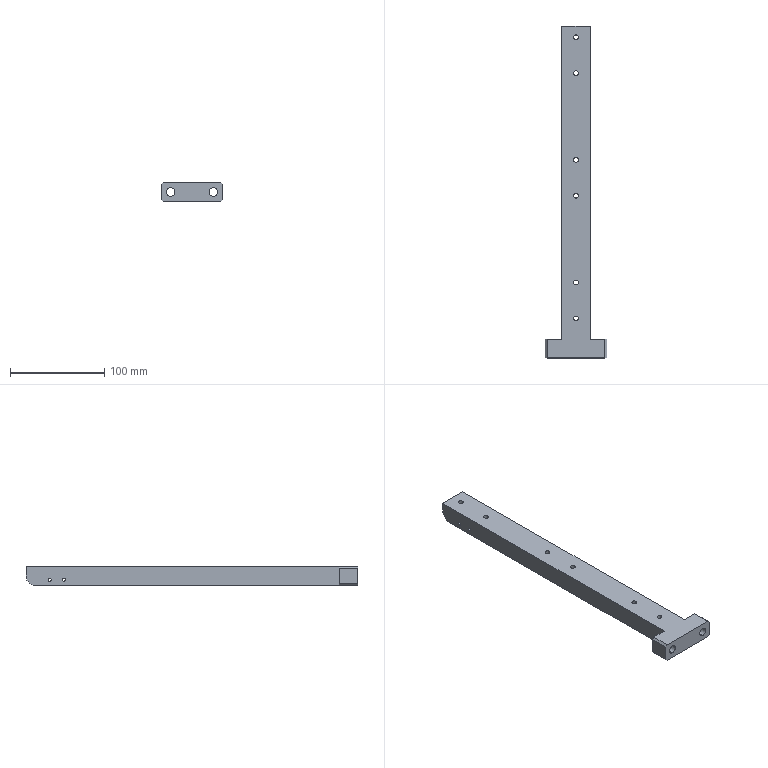Part | SolidWorks | features HoleWzd 3, Chamfer 1, Extrusion 1, Fillet 1, LPattern 1 | 1 solid | 35 faces | box 65 x 352 x 20 mm | volume 218982 mm3 | cylinder 21 | plane 14 | commonest cylinder face diameters 5 x12 3.3 x4 9 x4 20 x1
STEP:
#1=CARTESIAN_POINT('',(-2.5,302.,0.));
#2=VERTEX_POINT('',#1);
#3=CARTESIAN_POINT('',(2.5,302.,0.));
#4=VERTEX_POINT('',#3);
#5=CARTESIAN_POINT('',(0.,302.,0.));
#6=DIRECTION('',(0.,0.,1.));
#7=DIRECTION('',(1.,0.,0.));
#8=AXIS2_PLACEMENT_3D('',#5,#6,#7);
#9=CIRCLE('',#8,2.5);
#10=EDGE_CURVE('',#2,#4,#9,.T.);
#11=ORIENTED_EDGE('',*,*,#10,.F.);
#12=CARTESIAN_POINT('',(-2.5,302.,20.));
#13=VERTEX_POINT('',#12);
#14=CARTESIAN_POINT('',(-2.5,302.,20.));
#15=DIRECTION('',(0.,0.,1.));
#16=VECTOR('',#15,1000.);
#17=LINE('',#14,#16);
#18=EDGE_CURVE('',#2,#13,#17,.T.);
#19=ORIENTED_EDGE('',*,*,#18,.T.);
#20=CARTESIAN_POINT('',(2.5,302.,20.));
#21=VERTEX_POINT('',#20);
#22=CARTESIAN_POINT('',(0.,302.,20.));
#23=DIRECTION('',(0.,0.,1.));
#24=DIRECTION('',(1.,0.,0.));
#25=AXIS2_PLACEMENT_3D('',#22,#23,#24);
#26=CIRCLE('',#25,2.5);
#27=EDGE_CURVE('',#13,#21,#26,.T.);
#28=ORIENTED_EDGE('',*,*,#27,.T.);
#29=CARTESIAN_POINT('',(2.5,302.,20.));
#30=DIRECTION('',(0.,0.,1.));
#31=VECTOR('',#30,1000.);
#32=LINE('',#29,#31);
#33=EDGE_CURVE('',#4,#21,#32,.T.);
#34=ORIENTED_EDGE('',*,*,#33,.F.);
#35=EDGE_LOOP('',(#11,#19,#28,#34));
#36=FACE_OUTER_BOUND('',#35,.T.);
#37=CARTESIAN_POINT('',(0.,302.,20.));
#38=DIRECTION('',(0.,0.,1.));
#39=DIRECTION('',(1.,0.,0.));
#40=AXIS2_PLACEMENT_3D('',#37,#38,#39);
#41=CYLINDRICAL_SURFACE('',#40,2.5);
#42=ADVANCED_FACE('',(#36),#41,.F.);
#43=CARTESIAN_POINT('',(-2.5,172.,0.));
#44=VERTEX_POINT('',#43);
#45=CARTESIAN_POINT('',(2.5,172.,0.));
#46=VERTEX_POINT('',#45);
#47=CARTESIAN_POINT('',(0.,172.,0.));
#48=DIRECTION('',(0.,0.,1.));
#49=DIRECTION('',(1.,0.,0.));
#50=AXIS2_PLACEMENT_3D('',#47,#48,#49);
#51=CIRCLE('',#50,2.5);
#52=EDGE_CURVE('',#44,#46,#51,.T.);
#53=ORIENTED_EDGE('',*,*,#52,.F.);
#54=CARTESIAN_POINT('',(-2.5,172.,20.));
#55=VERTEX_POINT('',#54);
#56=CARTESIAN_POINT('',(-2.5,172.,20.));
#57=DIRECTION('',(0.,0.,1.));
#58=VECTOR('',#57,1000.);
#59=LINE('',#56,#58);
#60=EDGE_CURVE('',#44,#55,#59,.T.);
#61=ORIENTED_EDGE('',*,*,#60,.T.);
#62=CARTESIAN_POINT('',(2.5,172.,20.));
#63=VERTEX_POINT('',#62);
#64=CARTESIAN_POINT('',(0.,172.,20.));
#65=DIRECTION('',(0.,0.,1.));
#66=DIRECTION('',(1.,0.,0.));
#67=AXIS2_PLACEMENT_3D('',#64,#65,#66);
#68=CIRCLE('',#67,2.5);
#69=EDGE_CURVE('',#55,#63,#68,.T.);
#70=ORIENTED_EDGE('',*,*,#69,.T.);
#71=CARTESIAN_POINT('',(2.5,172.,20.));
#72=DIRECTION('',(0.,0.,1.));
#73=VECTOR('',#72,1000.);
#74=LINE('',#71,#73);
#75=EDGE_CURVE('',#46,#63,#74,.T.);
#76=ORIENTED_EDGE('',*,*,#75,.F.);
#77=EDGE_LOOP('',(#53,#61,#70,#76));
#78=FACE_OUTER_BOUND('',#77,.T.);
#79=CARTESIAN_POINT('',(0.,172.,20.));
#80=DIRECTION('',(0.,0.,1.));
#81=DIRECTION('',(1.,0.,0.));
#82=AXIS2_PLACEMENT_3D('',#79,#80,#81);
#83=CYLINDRICAL_SURFACE('',#82,2.5);
#84=ADVANCED_FACE('',(#78),#83,.F.);
#85=CARTESIAN_POINT('',(-2.5,42.,0.));
#86=VERTEX_POINT('',#85);
#87=CARTESIAN_POINT('',(2.5,42.,0.));
#88=VERTEX_POINT('',#87);
#89=CARTESIAN_POINT('',(0.,42.,0.));
#90=DIRECTION('',(0.,0.,1.));
#91=DIRECTION('',(1.,0.,0.));
#92=AXIS2_PLACEMENT_3D('',#89,#90,#91);
#93=CIRCLE('',#92,2.5);
#94=EDGE_CURVE('',#86,#88,#93,.T.);
#95=ORIENTED_EDGE('',*,*,#94,.F.);
#96=CARTESIAN_POINT('',(-2.5,42.,20.));
#97=VERTEX_POINT('',#96);
#98=CARTESIAN_POINT('',(-2.5,42.,20.));
#99=DIRECTION('',(0.,0.,1.));
#100=VECTOR('',#99,1000.);
#101=LINE('',#98,#100);
#102=EDGE_CURVE('',#86,#97,#101,.T.);
#103=ORIENTED_EDGE('',*,*,#102,.T.);
#104=CARTESIAN_POINT('',(2.5,42.,20.));
#105=VERTEX_POINT('',#104);
#106=CARTESIAN_POINT('',(0.,42.,20.));
#107=DIRECTION('',(0.,0.,1.));
#108=DIRECTION('',(1.,0.,0.));
#109=AXIS2_PLACEMENT_3D('',#106,#107,#108);
#110=CIRCLE('',#109,2.5);
#111=EDGE_CURVE('',#97,#105,#110,.T.);
#112=ORIENTED_EDGE('',*,*,#111,.T.);
#113=CARTESIAN_POINT('',(2.5,42.,20.));
#114=DIRECTION('',(0.,0.,1.));
#115=VECTOR('',#114,1000.);
#116=LINE('',#113,#115);
#117=EDGE_CURVE('',#88,#105,#116,.T.);
#118=ORIENTED_EDGE('',*,*,#117,.F.);
#119=EDGE_LOOP('',(#95,#103,#112,#118));
#120=FACE_OUTER_BOUND('',#119,.T.);
#121=CARTESIAN_POINT('',(0.,42.,20.));
#122=DIRECTION('',(0.,0.,1.));
#123=DIRECTION('',(1.,0.,0.));
#124=AXIS2_PLACEMENT_3D('',#121,#122,#123);
#125=CYLINDRICAL_SURFACE('',#124,2.5);
#126=ADVANCED_FACE('',(#120),#125,.F.);
#127=CARTESIAN_POINT('',(15.,327.,4.35));
#128=VERTEX_POINT('',#127);
#129=CARTESIAN_POINT('',(15.,327.,7.65));
#130=VERTEX_POINT('',#129);
#131=CARTESIAN_POINT('',(15.,327.,6.));
#132=DIRECTION('',(-1.,0.,0.));
#133=DIRECTION('',(0.,-1.,0.));
#134=AXIS2_PLACEMENT_3D('',#131,#132,#133);
#135=CIRCLE('',#134,1.65);
#136=EDGE_CURVE('',#128,#130,#135,.T.);
#137=ORIENTED_EDGE('',*,*,#136,.F.);
#138=CARTESIAN_POINT('',(-15.,327.,4.35));
#139=VERTEX_POINT('',#138);
#140=CARTESIAN_POINT('',(-15.,327.,4.35));
#141=DIRECTION('',(-1.,0.,0.));
#142=VECTOR('',#141,1000.);
#143=LINE('',#140,#142);
#144=EDGE_CURVE('',#128,#139,#143,.T.);
#145=ORIENTED_EDGE('',*,*,#144,.T.);
#146=CARTESIAN_POINT('',(-15.,327.,7.65));
#147=VERTEX_POINT('',#146);
#148=CARTESIAN_POINT('',(-15.,327.,6.));
#149=DIRECTION('',(-1.,0.,0.));
#150=DIRECTION('',(0.,0.,1.));
#151=AXIS2_PLACEMENT_3D('',#148,#149,#150);
#152=CIRCLE('',#151,1.65);
#153=EDGE_CURVE('',#139,#147,#152,.T.);
#154=ORIENTED_EDGE('',*,*,#153,.T.);
#155=CARTESIAN_POINT('',(-15.,327.,7.65));
#156=DIRECTION('',(-1.,0.,0.));
#157=VECTOR('',#156,1000.);
#158=LINE('',#155,#157);
#159=EDGE_CURVE('',#130,#147,#158,.T.);
#160=ORIENTED_EDGE('',*,*,#159,.F.);
#161=EDGE_LOOP('',(#137,#145,#154,#160));
#162=FACE_OUTER_BOUND('',#161,.T.);
#163=CARTESIAN_POINT('',(-15.,327.,6.));
#164=DIRECTION('',(-1.,0.,0.));
#165=DIRECTION('',(0.,0.,1.));
#166=AXIS2_PLACEMENT_3D('',#163,#164,#165);
#167=CYLINDRICAL_SURFACE('',#166,1.65);
#168=ADVANCED_FACE('',(#162),#167,.F.);
#169=CARTESIAN_POINT('',(15.,312.,4.35));
#170=VERTEX_POINT('',#169);
#171=CARTESIAN_POINT('',(15.,312.,7.65));
#172=VERTEX_POINT('',#171);
#173=CARTESIAN_POINT('',(15.,312.,6.));
#174=DIRECTION('',(-1.,0.,0.));
#175=DIRECTION('',(0.,-1.,0.));
#176=AXIS2_PLACEMENT_3D('',#173,#174,#175);
#177=CIRCLE('',#176,1.65);
#178=EDGE_CURVE('',#170,#172,#177,.T.);
#179=ORIENTED_EDGE('',*,*,#178,.F.);
#180=CARTESIAN_POINT('',(-15.,312.,4.35));
#181=VERTEX_POINT('',#180);
#182=CARTESIAN_POINT('',(-15.,312.,4.35));
#183=DIRECTION('',(-1.,0.,0.));
#184=VECTOR('',#183,1000.);
#185=LINE('',#182,#184);
#186=EDGE_CURVE('',#170,#181,#185,.T.);
#187=ORIENTED_EDGE('',*,*,#186,.T.);
#188=CARTESIAN_POINT('',(-15.,312.,7.65));
#189=VERTEX_POINT('',#188);
#190=CARTESIAN_POINT('',(-15.,312.,6.));
#191=DIRECTION('',(-1.,0.,0.));
#192=DIRECTION('',(0.,0.,1.));
#193=AXIS2_PLACEMENT_3D('',#190,#191,#192);
#194=CIRCLE('',#193,1.65);
#195=EDGE_CURVE('',#181,#189,#194,.T.);
#196=ORIENTED_EDGE('',*,*,#195,.T.);
#197=CARTESIAN_POINT('',(-15.,312.,7.65));
#198=DIRECTION('',(-1.,0.,0.));
#199=VECTOR('',#198,1000.);
#200=LINE('',#197,#199);
#201=EDGE_CURVE('',#172,#189,#200,.T.);
#202=ORIENTED_EDGE('',*,*,#201,.F.);
#203=EDGE_LOOP('',(#179,#187,#196,#202));
#204=FACE_OUTER_BOUND('',#203,.T.);
#205=CARTESIAN_POINT('',(-15.,312.,6.));
#206=DIRECTION('',(-1.,0.,0.));
#207=DIRECTION('',(0.,0.,1.));
#208=AXIS2_PLACEMENT_3D('',#205,#206,#207);
#209=CYLINDRICAL_SURFACE('',#208,1.65);
#210=ADVANCED_FACE('',(#204),#209,.F.);
#211=CARTESIAN_POINT('',(-2.5,340.,0.));
#212=VERTEX_POINT('',#211);
#213=CARTESIAN_POINT('',(2.5,340.,0.));
#214=VERTEX_POINT('',#213);
#215=CARTESIAN_POINT('',(0.,340.,0.));
#216=DIRECTION('',(0.,0.,1.));
#217=DIRECTION('',(1.,0.,0.));
#218=AXIS2_PLACEMENT_3D('',#215,#216,#217);
#219=CIRCLE('',#218,2.5);
#220=EDGE_CURVE('',#212,#214,#219,.T.);
#221=ORIENTED_EDGE('',*,*,#220,.F.);
#222=CARTESIAN_POINT('',(-2.5,340.,20.));
#223=VERTEX_POINT('',#222);
#224=CARTESIAN_POINT('',(-2.5,340.,20.));
#225=DIRECTION('',(0.,0.,1.));
#226=VECTOR('',#225,1000.);
#227=LINE('',#224,#226);
#228=EDGE_CURVE('',#212,#223,#227,.T.);
#229=ORIENTED_EDGE('',*,*,#228,.T.);
#230=CARTESIAN_POINT('',(2.5,340.,20.));
#231=VERTEX_POINT('',#230);
#232=CARTESIAN_POINT('',(0.,340.,20.));
#233=DIRECTION('',(0.,0.,1.));
#234=DIRECTION('',(1.,0.,0.));
#235=AXIS2_PLACEMENT_3D('',#232,#233,#234);
#236=CIRCLE('',#235,2.5);
#237=EDGE_CURVE('',#223,#231,#236,.T.);
#238=ORIENTED_EDGE('',*,*,#237,.T.);
#239=CARTESIAN_POINT('',(2.5,340.,20.));
#240=DIRECTION('',(0.,0.,1.));
#241=VECTOR('',#240,1000.);
#242=LINE('',#239,#241);
#243=EDGE_CURVE('',#214,#231,#242,.T.);
#244=ORIENTED_EDGE('',*,*,#243,.F.);
#245=EDGE_LOOP('',(#221,#229,#238,#244));
#246=FACE_OUTER_BOUND('',#245,.T.);
#247=CARTESIAN_POINT('',(0.,340.,20.));
#248=DIRECTION('',(0.,0.,1.));
#249=DIRECTION('',(1.,0.,0.));
#250=AXIS2_PLACEMENT_3D('',#247,#248,#249);
#251=CYLINDRICAL_SURFACE('',#250,2.5);
#252=ADVANCED_FACE('',(#246),#251,.F.);
#253=CARTESIAN_POINT('',(-2.5,210.,0.));
#254=VERTEX_POINT('',#253);
#255=CARTESIAN_POINT('',(2.5,210.,0.));
#256=VERTEX_POINT('',#255);
#257=CARTESIAN_POINT('',(0.,210.,0.));
#258=DIRECTION('',(0.,0.,1.));
#259=DIRECTION('',(1.,0.,0.));
#260=AXIS2_PLACEMENT_3D('',#257,#258,#259);
#261=CIRCLE('',#260,2.5);
#262=EDGE_CURVE('',#254,#256,#261,.T.);
#263=ORIENTED_EDGE('',*,*,#262,.F.);
#264=CARTESIAN_POINT('',(-2.5,210.,20.));
#265=VERTEX_POINT('',#264);
#266=CARTESIAN_POINT('',(-2.5,210.,20.));
#267=DIRECTION('',(0.,0.,1.));
#268=VECTOR('',#267,1000.);
#269=LINE('',#266,#268);
#270=EDGE_CURVE('',#254,#265,#269,.T.);
#271=ORIENTED_EDGE('',*,*,#270,.T.);
#272=CARTESIAN_POINT('',(2.5,210.,20.));
#273=VERTEX_POINT('',#272);
#274=CARTESIAN_POINT('',(0.,210.,20.));
#275=DIRECTION('',(0.,0.,1.));
#276=DIRECTION('',(1.,0.,0.));
#277=AXIS2_PLACEMENT_3D('',#274,#275,#276);
#278=CIRCLE('',#277,2.5);
#279=EDGE_CURVE('',#265,#273,#278,.T.);
#280=ORIENTED_EDGE('',*,*,#279,.T.);
#281=CARTESIAN_POINT('',(2.5,210.,20.));
#282=DIRECTION('',(0.,0.,1.));
#283=VECTOR('',#282,1000.);
#284=LINE('',#281,#283);
#285=EDGE_CURVE('',#256,#273,#284,.T.);
#286=ORIENTED_EDGE('',*,*,#285,.F.);
#287=EDGE_LOOP('',(#263,#271,#280,#286));
#288=FACE_OUTER_BOUND('',#287,.T.);
#289=CARTESIAN_POINT('',(0.,210.,20.));
#290=DIRECTION('',(0.,0.,1.));
#291=DIRECTION('',(1.,0.,0.));
#292=AXIS2_PLACEMENT_3D('',#289,#290,#291);
#293=CYLINDRICAL_SURFACE('',#292,2.5);
#294=ADVANCED_FACE('',(#288),#293,.F.);
#295=CARTESIAN_POINT('',(-2.5,80.,0.));
#296=VERTEX_POINT('',#295);
#297=CARTESIAN_POINT('',(2.5,80.,0.));
#298=VERTEX_POINT('',#297);
#299=CARTESIAN_POINT('',(0.,80.,0.));
#300=DIRECTION('',(0.,0.,1.));
#301=DIRECTION('',(1.,0.,0.));
#302=AXIS2_PLACEMENT_3D('',#299,#300,#301);
#303=CIRCLE('',#302,2.5);
#304=EDGE_CURVE('',#296,#298,#303,.T.);
#305=ORIENTED_EDGE('',*,*,#304,.F.);
#306=CARTESIAN_POINT('',(-2.5,80.,20.));
#307=VERTEX_POINT('',#306);
#308=CARTESIAN_POINT('',(-2.5,80.,20.));
#309=DIRECTION('',(0.,0.,1.));
#310=VECTOR('',#309,1000.);
#311=LINE('',#308,#310);
#312=EDGE_CURVE('',#296,#307,#311,.T.);
#313=ORIENTED_EDGE('',*,*,#312,.T.);
#314=CARTESIAN_POINT('',(2.5,80.,20.));
#315=VERTEX_POINT('',#314);
#316=CARTESIAN_POINT('',(0.,80.,20.));
#317=DIRECTION('',(0.,0.,1.));
#318=DIRECTION('',(1.,0.,0.));
#319=AXIS2_PLACEMENT_3D('',#316,#317,#318);
#320=CIRCLE('',#319,2.5);
#321=EDGE_CURVE('',#307,#315,#320,.T.);
#322=ORIENTED_EDGE('',*,*,#321,.T.);
#323=CARTESIAN_POINT('',(2.5,80.,20.));
#324=DIRECTION('',(0.,0.,1.));
#325=VECTOR('',#324,1000.);
#326=LINE('',#323,#325);
#327=EDGE_CURVE('',#298,#315,#326,.T.);
#328=ORIENTED_EDGE('',*,*,#327,.F.);
#329=EDGE_LOOP('',(#305,#313,#322,#328));
#330=FACE_OUTER_BOUND('',#329,.T.);
#331=CARTESIAN_POINT('',(0.,80.,20.));
#332=DIRECTION('',(0.,0.,1.));
#333=DIRECTION('',(1.,0.,0.));
#334=AXIS2_PLACEMENT_3D('',#331,#332,#333);
#335=CYLINDRICAL_SURFACE('',#334,2.5);
#336=ADVANCED_FACE('',(#330),#335,.F.);
#337=CARTESIAN_POINT('',(22.5,0.,5.5));
#338=VERTEX_POINT('',#337);
#339=CARTESIAN_POINT('',(22.5,0.,14.5));
#340=VERTEX_POINT('',#339);
#341=CARTESIAN_POINT('',(22.5,0.,10.));
#342=DIRECTION('',(0.,1.,0.));
#343=DIRECTION('',(0.,0.,1.));
#344=AXIS2_PLACEMENT_3D('',#341,#342,#343);
#345=CIRCLE('',#344,4.5);
#346=EDGE_CURVE('',#338,#340,#345,.T.);
#347=ORIENTED_EDGE('',*,*,#346,.F.);
#348=CARTESIAN_POINT('',(22.5,20.,5.5));
#349=VERTEX_POINT('',#348);
#350=CARTESIAN_POINT('',(22.5,20.,5.5));
#351=DIRECTION('',(0.,1.,0.));
#352=VECTOR('',#351,1000.);
#353=LINE('',#350,#352);
#354=EDGE_CURVE('',#338,#349,#353,.T.);
#355=ORIENTED_EDGE('',*,*,#354,.T.);
#356=CARTESIAN_POINT('',(22.5,20.,14.5));
#357=VERTEX_POINT('',#356);
#358=CARTESIAN_POINT('',(22.5,20.,10.));
#359=DIRECTION('',(0.,1.,0.));
#360=DIRECTION('',(0.,0.,1.));
#361=AXIS2_PLACEMENT_3D('',#358,#359,#360);
#362=CIRCLE('',#361,4.5);
#363=EDGE_CURVE('',#349,#357,#362,.T.);
#364=ORIENTED_EDGE('',*,*,#363,.T.);
#365=CARTESIAN_POINT('',(22.5,20.,14.5));
#366=DIRECTION('',(0.,1.,0.));
#367=VECTOR('',#366,1000.);
#368=LINE('',#365,#367);
#369=EDGE_CURVE('',#340,#357,#368,.T.);
#370=ORIENTED_EDGE('',*,*,#369,.F.);
#371=EDGE_LOOP('',(#347,#355,#364,#370));
#372=FACE_OUTER_BOUND('',#371,.T.);
#373=CARTESIAN_POINT('',(22.5,20.,10.));
#374=DIRECTION('',(0.,1.,0.));
#375=DIRECTION('',(0.,0.,1.));
#376=AXIS2_PLACEMENT_3D('',#373,#374,#375);
#377=CYLINDRICAL_SURFACE('',#376,4.5);
#378=ADVANCED_FACE('',(#372),#377,.F.);
#379=CARTESIAN_POINT('',(-22.5,0.,5.5));
#380=VERTEX_POINT('',#379);
#381=CARTESIAN_POINT('',(-22.5,0.,14.5));
#382=VERTEX_POINT('',#381);
#383=CARTESIAN_POINT('',(-22.5,0.,10.));
#384=DIRECTION('',(0.,1.,0.));
#385=DIRECTION('',(0.,0.,1.));
#386=AXIS2_PLACEMENT_3D('',#383,#384,#385);
#387=CIRCLE('',#386,4.5);
#388=EDGE_CURVE('',#380,#382,#387,.T.);
#389=ORIENTED_EDGE('',*,*,#388,.F.);
#390=CARTESIAN_POINT('',(-22.5,20.,5.5));
#391=VERTEX_POINT('',#390);
#392=CARTESIAN_POINT('',(-22.5,20.,5.5));
#393=DIRECTION('',(0.,1.,0.));
#394=VECTOR('',#393,1000.);
#395=LINE('',#392,#394);
#396=EDGE_CURVE('',#380,#391,#395,.T.);
#397=ORIENTED_EDGE('',*,*,#396,.T.);
#398=CARTESIAN_POINT('',(-22.5,20.,14.5));
#399=VERTEX_POINT('',#398);
#400=CARTESIAN_POINT('',(-22.5,20.,10.));
#401=DIRECTION('',(0.,1.,0.));
#402=DIRECTION('',(0.,0.,1.));
#403=AXIS2_PLACEMENT_3D('',#400,#401,#402);
#404=CIRCLE('',#403,4.5);
#405=EDGE_CURVE('',#391,#399,#404,.T.);
#406=ORIENTED_EDGE('',*,*,#405,.T.);
#407=CARTESIAN_POINT('',(-22.5,20.,14.5));
#408=DIRECTION('',(0.,1.,0.));
#409=VECTOR('',#408,1000.);
#410=LINE('',#407,#409);
#411=EDGE_CURVE('',#382,#399,#410,.T.);
#412=ORIENTED_EDGE('',*,*,#411,.F.);
#413=EDGE_LOOP('',(#389,#397,#406,#412));
#414=FACE_OUTER_BOUND('',#413,.T.);
#415=CARTESIAN_POINT('',(-22.5,20.,10.));
#416=DIRECTION('',(0.,1.,0.));
#417=DIRECTION('',(0.,0.,1.));
#418=AXIS2_PLACEMENT_3D('',#415,#416,#417);
#419=CYLINDRICAL_SURFACE('',#418,4.5);
#420=ADVANCED_FACE('',(#414),#419,.F.);
#421=CARTESIAN_POINT('',(0.,302.,0.));
#422=DIRECTION('',(0.,0.,1.));
#423=DIRECTION('',(1.,0.,0.));
#424=AXIS2_PLACEMENT_3D('',#421,#422,#423);
#425=CIRCLE('',#424,2.5);
#426=EDGE_CURVE('',#4,#2,#425,.T.);
#427=ORIENTED_EDGE('',*,*,#426,.T.);
#428=ORIENTED_EDGE('',*,*,#10,.T.);
#429=EDGE_LOOP('',(#427,#428));
#430=FACE_BOUND('',#429,.T.);
#431=CARTESIAN_POINT('',(0.,172.,0.));
#432=DIRECTION('',(0.,0.,1.));
#433=DIRECTION('',(1.,0.,0.));
#434=AXIS2_PLACEMENT_3D('',#431,#432,#433);
#435=CIRCLE('',#434,2.5);
#436=EDGE_CURVE('',#46,#44,#435,.T.);
#437=ORIENTED_EDGE('',*,*,#436,.T.);
#438=ORIENTED_EDGE('',*,*,#52,.T.);
#439=EDGE_LOOP('',(#437,#438));
#440=FACE_BOUND('',#439,.T.);
#441=CARTESIAN_POINT('',(0.,80.,0.));
#442=DIRECTION('',(0.,0.,1.));
#443=DIRECTION('',(1.,0.,0.));
#444=AXIS2_PLACEMENT_3D('',#441,#442,#443);
#445=CIRCLE('',#444,2.5);
#446=EDGE_CURVE('',#298,#296,#445,.T.);
#447=ORIENTED_EDGE('',*,*,#446,.T.);
#448=ORIENTED_EDGE('',*,*,#304,.T.);
#449=EDGE_LOOP('',(#447,#448));
#450=FACE_BOUND('',#449,.T.);
#451=CARTESIAN_POINT('',(0.,210.,0.));
#452=DIRECTION('',(0.,0.,1.));
#453=DIRECTION('',(1.,0.,0.));
#454=AXIS2_PLACEMENT_3D('',#451,#452,#453);
#455=CIRCLE('',#454,2.5);
#456=EDGE_CURVE('',#256,#254,#455,.T.);
#457=ORIENTED_EDGE('',*,*,#456,.T.);
#458=ORIENTED_EDGE('',*,*,#262,.T.);
#459=EDGE_LOOP('',(#457,#458));
#460=FACE_BOUND('',#459,.T.);
#461=CARTESIAN_POINT('',(30.5,20.,0.));
#462=VERTEX_POINT('',#461);
#463=CARTESIAN_POINT('',(15.,20.,0.));
#464=VERTEX_POINT('',#463);
#465=CARTESIAN_POINT('',(15.,20.,0.));
#466=DIRECTION('',(-1.,0.,0.));
#467=VECTOR('',#466,1000.);
#468=LINE('',#465,#467);
#469=EDGE_CURVE('',#462,#464,#468,.T.);
#470=ORIENTED_EDGE('',*,*,#469,.F.);
#471=CARTESIAN_POINT('',(30.5,0.,0.));
#472=VERTEX_POINT('',#471);
#473=CARTESIAN_POINT('',(30.5,0.,0.));
#474=DIRECTION('',(0.,-1.,0.));
#475=VECTOR('',#474,1000.);
#476=LINE('',#473,#475);
#477=EDGE_CURVE('',#462,#472,#476,.T.);
#478=ORIENTED_EDGE('',*,*,#477,.T.);
#479=CARTESIAN_POINT('',(-30.5,0.,0.));
#480=VERTEX_POINT('',#479);
#481=CARTESIAN_POINT('',(-32.5,0.,0.));
#482=DIRECTION('',(1.,0.,0.));
#483=VECTOR('',#482,1000.);
#484=LINE('',#481,#483);
#485=EDGE_CURVE('',#480,#472,#484,.T.);
#486=ORIENTED_EDGE('',*,*,#485,.F.);
#487=CARTESIAN_POINT('',(-30.5,20.,0.));
#488=VERTEX_POINT('',#487);
#489=CARTESIAN_POINT('',(-30.5,20.,0.));
#490=DIRECTION('',(0.,1.,0.));
#491=VECTOR('',#490,1000.);
#492=LINE('',#489,#491);
#493=EDGE_CURVE('',#480,#488,#492,.T.);
#494=ORIENTED_EDGE('',*,*,#493,.T.);
#495=CARTESIAN_POINT('',(-15.,20.,0.));
#496=VERTEX_POINT('',#495);
#497=CARTESIAN_POINT('',(-15.,20.,0.));
#498=DIRECTION('',(-1.,0.,0.));
#499=VECTOR('',#498,1000.);
#500=LINE('',#497,#499);
#501=EDGE_CURVE('',#496,#488,#500,.T.);
#502=ORIENTED_EDGE('',*,*,#501,.F.);
#503=CARTESIAN_POINT('',(-15.,342.,0.));
#504=VERTEX_POINT('',#503);
#505=CARTESIAN_POINT('',(-15.,352.,0.));
#506=DIRECTION('',(0.,-1.,0.));
#507=VECTOR('',#506,1000.);
#508=LINE('',#505,#507);
#509=EDGE_CURVE('',#504,#496,#508,.T.);
#510=ORIENTED_EDGE('',*,*,#509,.F.);
#511=CARTESIAN_POINT('',(-1.5,342.,0.));
#512=VERTEX_POINT('',#511);
#513=CARTESIAN_POINT('',(15.,342.,0.));
#514=DIRECTION('',(1.,0.,0.));
#515=VECTOR('',#514,1000.);
#516=LINE('',#513,#515);
#517=EDGE_CURVE('',#504,#512,#516,.T.);
#518=ORIENTED_EDGE('',*,*,#517,.T.);
#519=CARTESIAN_POINT('',(0.,340.,0.));
#520=DIRECTION('',(0.,0.,1.));
#521=DIRECTION('',(1.,0.,0.));
#522=AXIS2_PLACEMENT_3D('',#519,#520,#521);
#523=CIRCLE('',#522,2.5);
#524=EDGE_CURVE('',#512,#212,#523,.T.);
#525=ORIENTED_EDGE('',*,*,#524,.T.);
#526=ORIENTED_EDGE('',*,*,#220,.T.);
#527=CARTESIAN_POINT('',(1.5,342.,0.));
#528=VERTEX_POINT('',#527);
#529=CARTESIAN_POINT('',(0.,340.,0.));
#530=DIRECTION('',(0.,0.,1.));
#531=DIRECTION('',(1.,0.,0.));
#532=AXIS2_PLACEMENT_3D('',#529,#530,#531);
#533=CIRCLE('',#532,2.5);
#534=EDGE_CURVE('',#214,#528,#533,.T.);
#535=ORIENTED_EDGE('',*,*,#534,.T.);
#536=CARTESIAN_POINT('',(15.,342.,0.));
#537=VERTEX_POINT('',#536);
#538=CARTESIAN_POINT('',(15.,342.,0.));
#539=DIRECTION('',(1.,0.,0.));
#540=VECTOR('',#539,1000.);
#541=LINE('',#538,#540);
#542=EDGE_CURVE('',#528,#537,#541,.T.);
#543=ORIENTED_EDGE('',*,*,#542,.T.);
#544=CARTESIAN_POINT('',(15.,352.,0.));
#545=DIRECTION('',(0.,1.,0.));
#546=VECTOR('',#545,1000.);
#547=LINE('',#544,#546);
#548=EDGE_CURVE('',#464,#537,#547,.T.);
#549=ORIENTED_EDGE('',*,*,#548,.F.);
#550=EDGE_LOOP('',(#470,#478,#486,#494,#502,#510,#518,#525,#526,#535,#543,#549));
#551=FACE_OUTER_BOUND('',#550,.T.);
#552=CARTESIAN_POINT('',(0.,42.,0.));
#553=DIRECTION('',(0.,0.,1.));
#554=DIRECTION('',(1.,0.,0.));
#555=AXIS2_PLACEMENT_3D('',#552,#553,#554);
#556=CIRCLE('',#555,2.5);
#557=EDGE_CURVE('',#88,#86,#556,.T.);
#558=ORIENTED_EDGE('',*,*,#557,.T.);
#559=ORIENTED_EDGE('',*,*,#94,.T.);
#560=EDGE_LOOP('',(#558,#559));
#561=FACE_BOUND('',#560,.T.);
#562=CARTESIAN_POINT('',(0.,0.,0.));
#563=DIRECTION('',(0.,0.,-1.));
#564=DIRECTION('',(-1.,0.,0.));
#565=AXIS2_PLACEMENT_3D('',#562,#563,#564);
#566=PLANE('',#565);
#567=ADVANCED_FACE('',(#430,#440,#450,#460,#551,#561),#566,.T.);
#568=CARTESIAN_POINT('',(-15.,327.,6.));
#569=DIRECTION('',(-1.,0.,0.));
#570=DIRECTION('',(0.,0.,1.));
#571=AXIS2_PLACEMENT_3D('',#568,#569,#570);
#572=CIRCLE('',#571,1.65);
#573=EDGE_CURVE('',#147,#139,#572,.T.);
#574=ORIENTED_EDGE('',*,*,#573,.F.);
#575=ORIENTED_EDGE('',*,*,#153,.F.);
#576=EDGE_LOOP('',(#574,#575));
#577=FACE_BOUND('',#576,.T.);
#578=CARTESIAN_POINT('',(-15.,312.,6.));
#579=DIRECTION('',(-1.,0.,0.));
#580=DIRECTION('',(0.,0.,1.));
#581=AXIS2_PLACEMENT_3D('',#578,#579,#580);
#582=CIRCLE('',#581,1.65);
#583=EDGE_CURVE('',#189,#181,#582,.T.);
#584=ORIENTED_EDGE('',*,*,#583,.F.);
#585=ORIENTED_EDGE('',*,*,#195,.F.);
#586=EDGE_LOOP('',(#584,#585));
#587=FACE_BOUND('',#586,.T.);
#588=CARTESIAN_POINT('',(-15.,352.,20.));
#589=VERTEX_POINT('',#588);
#590=CARTESIAN_POINT('',(-15.,352.,10.));
#591=VERTEX_POINT('',#590);
#592=CARTESIAN_POINT('',(-15.,352.,20.));
#593=DIRECTION('',(0.,0.,-1.));
#594=VECTOR('',#593,1000.);
#595=LINE('',#592,#594);
#596=EDGE_CURVE('',#589,#591,#595,.T.);
#597=ORIENTED_EDGE('',*,*,#596,.T.);
#598=CARTESIAN_POINT('',(-15.,342.,10.));
#599=DIRECTION('',(-1.,0.,0.));
#600=DIRECTION('',(0.,1.,0.));
#601=AXIS2_PLACEMENT_3D('',#598,#599,#600);
#602=CIRCLE('',#601,10.);
#603=EDGE_CURVE('',#591,#504,#602,.T.);
#604=ORIENTED_EDGE('',*,*,#603,.T.);
#605=ORIENTED_EDGE('',*,*,#509,.T.);
#606=CARTESIAN_POINT('',(-15.,20.,20.));
#607=VERTEX_POINT('',#606);
#608=CARTESIAN_POINT('',(-15.,20.,20.));
#609=DIRECTION('',(0.,0.,-1.));
#610=VECTOR('',#609,1000.);
#611=LINE('',#608,#610);
#612=EDGE_CURVE('',#607,#496,#611,.T.);
#613=ORIENTED_EDGE('',*,*,#612,.F.);
#614=CARTESIAN_POINT('',(-15.,352.,20.));
#615=DIRECTION('',(0.,-1.,0.));
#616=VECTOR('',#615,1000.);
#617=LINE('',#614,#616);
#618=EDGE_CURVE('',#589,#607,#617,.T.);
#619=ORIENTED_EDGE('',*,*,#618,.F.);
#620=EDGE_LOOP('',(#597,#604,#605,#613,#619));
#621=FACE_OUTER_BOUND('',#620,.T.);
#622=CARTESIAN_POINT('',(-15.,352.,20.));
#623=DIRECTION('',(1.,0.,0.));
#624=DIRECTION('',(0.,1.,0.));
#625=AXIS2_PLACEMENT_3D('',#622,#623,#624);
#626=PLANE('',#625);
#627=ADVANCED_FACE('',(#577,#587,#621),#626,.F.);
#628=CARTESIAN_POINT('',(-22.5,20.,10.));
#629=DIRECTION('',(0.,1.,0.));
#630=DIRECTION('',(0.,0.,1.));
#631=AXIS2_PLACEMENT_3D('',#628,#629,#630);
#632=CIRCLE('',#631,4.5);
#633=EDGE_CURVE('',#399,#391,#632,.T.);
#634=ORIENTED_EDGE('',*,*,#633,.F.);
#635=ORIENTED_EDGE('',*,*,#405,.F.);
#636=EDGE_LOOP('',(#634,#635));
#637=FACE_BOUND('',#636,.T.);
#638=CARTESIAN_POINT('',(-32.5,20.,18.));
#639=VERTEX_POINT('',#638);
#640=CARTESIAN_POINT('',(-32.5,20.,2.));
#641=VERTEX_POINT('',#640);
#642=CARTESIAN_POINT('',(-32.5,20.,20.));
#643=DIRECTION('',(0.,0.,-1.));
#644=VECTOR('',#643,1000.);
#645=LINE('',#642,#644);
#646=EDGE_CURVE('',#639,#641,#645,.T.);
#647=ORIENTED_EDGE('',*,*,#646,.F.);
#648=CARTESIAN_POINT('',(-30.5,20.,20.));
#649=VERTEX_POINT('',#648);
#650=CARTESIAN_POINT('',(-30.5,20.,20.));
#651=DIRECTION('',(0.7071,0.,0.7071));
#652=VECTOR('',#651,1000.);
#653=LINE('',#650,#652);
#654=EDGE_CURVE('',#639,#649,#653,.T.);
#655=ORIENTED_EDGE('',*,*,#654,.T.);
#656=CARTESIAN_POINT('',(-15.,20.,20.));
#657=DIRECTION('',(-1.,0.,0.));
#658=VECTOR('',#657,1000.);
#659=LINE('',#656,#658);
#660=EDGE_CURVE('',#607,#649,#659,.T.);
#661=ORIENTED_EDGE('',*,*,#660,.F.);
#662=ORIENTED_EDGE('',*,*,#612,.T.);
#663=ORIENTED_EDGE('',*,*,#501,.T.);
#664=CARTESIAN_POINT('',(-32.5,20.,2.));
#665=DIRECTION('',(-0.7071,0.,0.7071));
#666=VECTOR('',#665,1000.);
#667=LINE('',#664,#666);
#668=EDGE_CURVE('',#488,#641,#667,.T.);
#669=ORIENTED_EDGE('',*,*,#668,.T.);
#670=EDGE_LOOP('',(#647,#655,#661,#662,#663,#669));
#671=FACE_OUTER_BOUND('',#670,.T.);
#672=CARTESIAN_POINT('',(-15.,20.,20.));
#673=DIRECTION('',(0.,-1.,0.));
#674=DIRECTION('',(1.,0.,0.));
#675=AXIS2_PLACEMENT_3D('',#672,#673,#674);
#676=PLANE('',#675);
#677=ADVANCED_FACE('',(#637,#671),#676,.F.);
#678=CARTESIAN_POINT('',(-32.5,0.,18.));
#679=VERTEX_POINT('',#678);
#680=CARTESIAN_POINT('',(-32.5,0.,2.));
#681=VERTEX_POINT('',#680);
#682=CARTESIAN_POINT('',(-32.5,0.,20.));
#683=DIRECTION('',(0.,0.,-1.));
#684=VECTOR('',#683,1000.);
#685=LINE('',#682,#684);
#686=EDGE_CURVE('',#679,#681,#685,.T.);
#687=ORIENTED_EDGE('',*,*,#686,.F.);
#688=CARTESIAN_POINT('',(-32.5,20.,18.));
#689=DIRECTION('',(0.,1.,0.));
#690=VECTOR('',#689,1000.);
#691=LINE('',#688,#690);
#692=EDGE_CURVE('',#679,#639,#691,.T.);
#693=ORIENTED_EDGE('',*,*,#692,.T.);
#694=ORIENTED_EDGE('',*,*,#646,.T.);
#695=CARTESIAN_POINT('',(-32.5,0.,2.));
#696=DIRECTION('',(0.,-1.,0.));
#697=VECTOR('',#696,1000.);
#698=LINE('',#695,#697);
#699=EDGE_CURVE('',#641,#681,#698,.T.);
#700=ORIENTED_EDGE('',*,*,#699,.T.);
#701=EDGE_LOOP('',(#687,#693,#694,#700));
#702=FACE_OUTER_BOUND('',#701,.T.);
#703=CARTESIAN_POINT('',(-32.5,20.,20.));
#704=DIRECTION('',(1.,0.,0.));
#705=DIRECTION('',(0.,1.,0.));
#706=AXIS2_PLACEMENT_3D('',#703,#704,#705);
#707=PLANE('',#706);
#708=ADVANCED_FACE('',(#702),#707,.F.);
#709=CARTESIAN_POINT('',(22.5,0.,10.));
#710=DIRECTION('',(0.,1.,0.));
#711=DIRECTION('',(0.,0.,1.));
#712=AXIS2_PLACEMENT_3D('',#709,#710,#711);
#713=CIRCLE('',#712,4.5);
#714=EDGE_CURVE('',#340,#338,#713,.T.);
#715=ORIENTED_EDGE('',*,*,#714,.T.);
#716=ORIENTED_EDGE('',*,*,#346,.T.);
#717=EDGE_LOOP('',(#715,#716));
#718=FACE_BOUND('',#717,.T.);
#719=CARTESIAN_POINT('',(-22.5,0.,10.));
#720=DIRECTION('',(0.,1.,0.));
#721=DIRECTION('',(0.,0.,1.));
#722=AXIS2_PLACEMENT_3D('',#719,#720,#721);
#723=CIRCLE('',#722,4.5);
#724=EDGE_CURVE('',#382,#380,#723,.T.);
#725=ORIENTED_EDGE('',*,*,#724,.T.);
#726=ORIENTED_EDGE('',*,*,#388,.T.);
#727=EDGE_LOOP('',(#725,#726));
#728=FACE_BOUND('',#727,.T.);
#729=CARTESIAN_POINT('',(32.5,0.,18.));
#730=VERTEX_POINT('',#729);
#731=CARTESIAN_POINT('',(32.5,0.,2.));
#732=VERTEX_POINT('',#731);
#733=CARTESIAN_POINT('',(32.5,0.,20.));
#734=DIRECTION('',(0.,0.,-1.));
#735=VECTOR('',#734,1000.);
#736=LINE('',#733,#735);
#737=EDGE_CURVE('',#730,#732,#736,.T.);
#738=ORIENTED_EDGE('',*,*,#737,.F.);
#739=CARTESIAN_POINT('',(30.5,0.,20.));
#740=VERTEX_POINT('',#739);
#741=CARTESIAN_POINT('',(30.5,0.,20.));
#742=DIRECTION('',(-0.7071,0.,0.7071));
#743=VECTOR('',#742,1000.);
#744=LINE('',#741,#743);
#745=EDGE_CURVE('',#730,#740,#744,.T.);
#746=ORIENTED_EDGE('',*,*,#745,.T.);
#747=CARTESIAN_POINT('',(-30.5,0.,20.));
#748=VERTEX_POINT('',#747);
#749=CARTESIAN_POINT('',(-32.5,0.,20.));
#750=DIRECTION('',(1.,0.,0.));
#751=VECTOR('',#750,1000.);
#752=LINE('',#749,#751);
#753=EDGE_CURVE('',#748,#740,#752,.T.);
#754=ORIENTED_EDGE('',*,*,#753,.F.);
#755=CARTESIAN_POINT('',(-30.5,0.,20.));
#756=DIRECTION('',(-0.7071,0.,-0.7071));
#757=VECTOR('',#756,1000.);
#758=LINE('',#755,#757);
#759=EDGE_CURVE('',#748,#679,#758,.T.);
#760=ORIENTED_EDGE('',*,*,#759,.T.);
#761=ORIENTED_EDGE('',*,*,#686,.T.);
#762=CARTESIAN_POINT('',(-32.5,0.,2.));
#763=DIRECTION('',(0.7071,0.,-0.7071));
#764=VECTOR('',#763,1000.);
#765=LINE('',#762,#764);
#766=EDGE_CURVE('',#681,#480,#765,.T.);
#767=ORIENTED_EDGE('',*,*,#766,.T.);
#768=ORIENTED_EDGE('',*,*,#485,.T.);
#769=CARTESIAN_POINT('',(32.5,0.,2.));
#770=DIRECTION('',(0.7071,0.,0.7071));
#771=VECTOR('',#770,1000.);
#772=LINE('',#769,#771);
#773=EDGE_CURVE('',#472,#732,#772,.T.);
#774=ORIENTED_EDGE('',*,*,#773,.T.);
#775=EDGE_LOOP('',(#738,#746,#754,#760,#761,#767,#768,#774));
#776=FACE_OUTER_BOUND('',#775,.T.);
#777=CARTESIAN_POINT('',(-32.5,0.,20.));
#778=DIRECTION('',(0.,1.,0.));
#779=DIRECTION('',(0.,0.,1.));
#780=AXIS2_PLACEMENT_3D('',#777,#778,#779);
#781=PLANE('',#780);
#782=ADVANCED_FACE('',(#718,#728,#776),#781,.F.);
#783=CARTESIAN_POINT('',(32.5,20.,18.));
#784=VERTEX_POINT('',#783);
#785=CARTESIAN_POINT('',(32.5,20.,2.));
#786=VERTEX_POINT('',#785);
#787=CARTESIAN_POINT('',(32.5,20.,20.));
#788=DIRECTION('',(0.,0.,-1.));
#789=VECTOR('',#788,1000.);
#790=LINE('',#787,#789);
#791=EDGE_CURVE('',#784,#786,#790,.T.);
#792=ORIENTED_EDGE('',*,*,#791,.F.);
#793=CARTESIAN_POINT('',(32.5,20.,18.));
#794=DIRECTION('',(0.,-1.,0.));
#795=VECTOR('',#794,1000.);
#796=LINE('',#793,#795);
#797=EDGE_CURVE('',#784,#730,#796,.T.);
#798=ORIENTED_EDGE('',*,*,#797,.T.);
#799=ORIENTED_EDGE('',*,*,#737,.T.);
#800=CARTESIAN_POINT('',(32.5,20.,2.));
#801=DIRECTION('',(0.,1.,0.));
#802=VECTOR('',#801,1000.);
#803=LINE('',#800,#802);
#804=EDGE_CURVE('',#732,#786,#803,.T.);
#805=ORIENTED_EDGE('',*,*,#804,.T.);
#806=EDGE_LOOP('',(#792,#798,#799,#805));
#807=FACE_OUTER_BOUND('',#806,.T.);
#808=CARTESIAN_POINT('',(32.5,20.,20.));
#809=DIRECTION('',(-1.,0.,0.));
#810=DIRECTION('',(0.,-1.,0.));
#811=AXIS2_PLACEMENT_3D('',#808,#809,#810);
#812=PLANE('',#811);
#813=ADVANCED_FACE('',(#807),#812,.F.);
#814=CARTESIAN_POINT('',(22.5,20.,10.));
#815=DIRECTION('',(0.,1.,0.));
#816=DIRECTION('',(0.,0.,1.));
#817=AXIS2_PLACEMENT_3D('',#814,#815,#816);
#818=CIRCLE('',#817,4.5);
#819=EDGE_CURVE('',#357,#349,#818,.T.);
#820=ORIENTED_EDGE('',*,*,#819,.F.);
#821=ORIENTED_EDGE('',*,*,#363,.F.);
#822=EDGE_LOOP('',(#820,#821));
#823=FACE_BOUND('',#822,.T.);
#824=CARTESIAN_POINT('',(30.5,20.,20.));
#825=VERTEX_POINT('',#824);
#826=CARTESIAN_POINT('',(15.,20.,20.));
#827=VERTEX_POINT('',#826);
#828=CARTESIAN_POINT('',(15.,20.,20.));
#829=DIRECTION('',(-1.,0.,0.));
#830=VECTOR('',#829,1000.);
#831=LINE('',#828,#830);
#832=EDGE_CURVE('',#825,#827,#831,.T.);
#833=ORIENTED_EDGE('',*,*,#832,.F.);
#834=CARTESIAN_POINT('',(30.5,20.,20.));
#835=DIRECTION('',(0.7071,0.,-0.7071));
#836=VECTOR('',#835,1000.);
#837=LINE('',#834,#836);
#838=EDGE_CURVE('',#825,#784,#837,.T.);
#839=ORIENTED_EDGE('',*,*,#838,.T.);
#840=ORIENTED_EDGE('',*,*,#791,.T.);
#841=CARTESIAN_POINT('',(32.5,20.,2.));
#842=DIRECTION('',(-0.7071,0.,-0.7071));
#843=VECTOR('',#842,1000.);
#844=LINE('',#841,#843);
#845=EDGE_CURVE('',#786,#462,#844,.T.);
#846=ORIENTED_EDGE('',*,*,#845,.T.);
#847=ORIENTED_EDGE('',*,*,#469,.T.);
#848=CARTESIAN_POINT('',(15.,20.,20.));
#849=DIRECTION('',(0.,0.,-1.));
#850=VECTOR('',#849,1000.);
#851=LINE('',#848,#850);
#852=EDGE_CURVE('',#827,#464,#851,.T.);
#853=ORIENTED_EDGE('',*,*,#852,.F.);
#854=EDGE_LOOP('',(#833,#839,#840,#846,#847,#853));
#855=FACE_OUTER_BOUND('',#854,.T.);
#856=CARTESIAN_POINT('',(15.,20.,20.));
#857=DIRECTION('',(0.,-1.,0.));
#858=DIRECTION('',(1.,0.,0.));
#859=AXIS2_PLACEMENT_3D('',#856,#857,#858);
#860=PLANE('',#859);
#861=ADVANCED_FACE('',(#823,#855),#860,.F.);
#862=CARTESIAN_POINT('',(15.,327.,6.));
#863=DIRECTION('',(-1.,0.,0.));
#864=DIRECTION('',(0.,-1.,0.));
#865=AXIS2_PLACEMENT_3D('',#862,#863,#864);
#866=CIRCLE('',#865,1.65);
#867=EDGE_CURVE('',#130,#128,#866,.T.);
#868=ORIENTED_EDGE('',*,*,#867,.T.);
#869=ORIENTED_EDGE('',*,*,#136,.T.);
#870=EDGE_LOOP('',(#868,#869));
#871=FACE_BOUND('',#870,.T.);
#872=CARTESIAN_POINT('',(15.,312.,6.));
#873=DIRECTION('',(-1.,0.,0.));
#874=DIRECTION('',(0.,-1.,0.));
#875=AXIS2_PLACEMENT_3D('',#872,#873,#874);
#876=CIRCLE('',#875,1.65);
#877=EDGE_CURVE('',#172,#170,#876,.T.);
#878=ORIENTED_EDGE('',*,*,#877,.T.);
#879=ORIENTED_EDGE('',*,*,#178,.T.);
#880=EDGE_LOOP('',(#878,#879));
#881=FACE_BOUND('',#880,.T.);
#882=ORIENTED_EDGE('',*,*,#548,.T.);
#883=CARTESIAN_POINT('',(15.,352.,10.));
#884=VERTEX_POINT('',#883);
#885=CARTESIAN_POINT('',(15.,342.,10.));
#886=DIRECTION('',(1.,0.,0.));
#887=DIRECTION('',(0.,-1.,0.));
#888=AXIS2_PLACEMENT_3D('',#885,#886,#887);
#889=CIRCLE('',#888,10.);
#890=EDGE_CURVE('',#537,#884,#889,.T.);
#891=ORIENTED_EDGE('',*,*,#890,.T.);
#892=CARTESIAN_POINT('',(15.,352.,20.));
#893=VERTEX_POINT('',#892);
#894=CARTESIAN_POINT('',(15.,352.,20.));
#895=DIRECTION('',(0.,0.,-1.));
#896=VECTOR('',#895,1000.);
#897=LINE('',#894,#896);
#898=EDGE_CURVE('',#893,#884,#897,.T.);
#899=ORIENTED_EDGE('',*,*,#898,.F.);
#900=CARTESIAN_POINT('',(15.,352.,20.));
#901=DIRECTION('',(0.,1.,0.));
#902=VECTOR('',#901,1000.);
#903=LINE('',#900,#902);
#904=EDGE_CURVE('',#827,#893,#903,.T.);
#905=ORIENTED_EDGE('',*,*,#904,.F.);
#906=ORIENTED_EDGE('',*,*,#852,.T.);
#907=EDGE_LOOP('',(#882,#891,#899,#905,#906));
#908=FACE_OUTER_BOUND('',#907,.T.);
#909=CARTESIAN_POINT('',(15.,352.,20.));
#910=DIRECTION('',(-1.,0.,0.));
#911=DIRECTION('',(0.,-1.,0.));
#912=AXIS2_PLACEMENT_3D('',#909,#910,#911);
#913=PLANE('',#912);
#914=ADVANCED_FACE('',(#871,#881,#908),#913,.F.);
#915=ORIENTED_EDGE('',*,*,#898,.T.);
#916=CARTESIAN_POINT('',(-15.,352.,10.));
#917=DIRECTION('',(-1.,0.,0.));
#918=VECTOR('',#917,1000.);
#919=LINE('',#916,#918);
#920=EDGE_CURVE('',#884,#591,#919,.T.);
#921=ORIENTED_EDGE('',*,*,#920,.T.);
#922=ORIENTED_EDGE('',*,*,#596,.F.);
#923=CARTESIAN_POINT('',(15.,352.,20.));
#924=DIRECTION('',(-1.,0.,0.));
#925=VECTOR('',#924,1000.);
#926=LINE('',#923,#925);
#927=EDGE_CURVE('',#893,#589,#926,.T.);
#928=ORIENTED_EDGE('',*,*,#927,.F.);
#929=EDGE_LOOP('',(#915,#921,#922,#928));
#930=FACE_OUTER_BOUND('',#929,.T.);
#931=CARTESIAN_POINT('',(15.,352.,20.));
#932=DIRECTION('',(0.,-1.,0.));
#933=DIRECTION('',(0.,0.,-1.));
#934=AXIS2_PLACEMENT_3D('',#931,#932,#933);
#935=PLANE('',#934);
#936=ADVANCED_FACE('',(#930),#935,.F.);
#937=CARTESIAN_POINT('',(0.,302.,20.));
#938=DIRECTION('',(0.,0.,1.));
#939=DIRECTION('',(1.,0.,0.));
#940=AXIS2_PLACEMENT_3D('',#937,#938,#939);
#941=CIRCLE('',#940,2.5);
#942=EDGE_CURVE('',#21,#13,#941,.T.);
#943=ORIENTED_EDGE('',*,*,#942,.F.);
#944=ORIENTED_EDGE('',*,*,#27,.F.);
#945=EDGE_LOOP('',(#943,#944));
#946=FACE_BOUND('',#945,.T.);
#947=CARTESIAN_POINT('',(0.,172.,20.));
#948=DIRECTION('',(0.,0.,1.));
#949=DIRECTION('',(1.,0.,0.));
#950=AXIS2_PLACEMENT_3D('',#947,#948,#949);
#951=CIRCLE('',#950,2.5);
#952=EDGE_CURVE('',#63,#55,#951,.T.);
#953=ORIENTED_EDGE('',*,*,#952,.F.);
#954=ORIENTED_EDGE('',*,*,#69,.F.);
#955=EDGE_LOOP('',(#953,#954));
#956=FACE_BOUND('',#955,.T.);
#957=CARTESIAN_POINT('',(0.,42.,20.));
#958=DIRECTION('',(0.,0.,1.));
#959=DIRECTION('',(1.,0.,0.));
#960=AXIS2_PLACEMENT_3D('',#957,#958,#959);
#961=CIRCLE('',#960,2.5);
#962=EDGE_CURVE('',#105,#97,#961,.T.);
#963=ORIENTED_EDGE('',*,*,#962,.F.);
#964=ORIENTED_EDGE('',*,*,#111,.F.);
#965=EDGE_LOOP('',(#963,#964));
#966=FACE_BOUND('',#965,.T.);
#967=CARTESIAN_POINT('',(0.,340.,20.));
#968=DIRECTION('',(0.,0.,1.));
#969=DIRECTION('',(1.,0.,0.));
#970=AXIS2_PLACEMENT_3D('',#967,#968,#969);
#971=CIRCLE('',#970,2.5);
#972=EDGE_CURVE('',#231,#223,#971,.T.);
#973=ORIENTED_EDGE('',*,*,#972,.F.);
#974=ORIENTED_EDGE('',*,*,#237,.F.);
#975=EDGE_LOOP('',(#973,#974));
#976=FACE_BOUND('',#975,.T.);
#977=CARTESIAN_POINT('',(0.,210.,20.));
#978=DIRECTION('',(0.,0.,1.));
#979=DIRECTION('',(1.,0.,0.));
#980=AXIS2_PLACEMENT_3D('',#977,#978,#979);
#981=CIRCLE('',#980,2.5);
#982=EDGE_CURVE('',#273,#265,#981,.T.);
#983=ORIENTED_EDGE('',*,*,#982,.F.);
#984=ORIENTED_EDGE('',*,*,#279,.F.);
#985=EDGE_LOOP('',(#983,#984));
#986=FACE_BOUND('',#985,.T.);
#987=CARTESIAN_POINT('',(0.,80.,20.));
#988=DIRECTION('',(0.,0.,1.));
#989=DIRECTION('',(1.,0.,0.));
#990=AXIS2_PLACEMENT_3D('',#987,#988,#989);
#991=CIRCLE('',#990,2.5);
#992=EDGE_CURVE('',#315,#307,#991,.T.);
#993=ORIENTED_EDGE('',*,*,#992,.F.);
#994=ORIENTED_EDGE('',*,*,#321,.F.);
#995=EDGE_LOOP('',(#993,#994));
#996=FACE_BOUND('',#995,.T.);
#997=ORIENTED_EDGE('',*,*,#753,.T.);
#998=CARTESIAN_POINT('',(30.5,0.,20.));
#999=DIRECTION('',(0.,1.,0.));
#1000=VECTOR('',#999,1000.);
#1001=LINE('',#998,#1000);
#1002=EDGE_CURVE('',#740,#825,#1001,.T.);
#1003=ORIENTED_EDGE('',*,*,#1002,.T.);
#1004=ORIENTED_EDGE('',*,*,#832,.T.);
#1005=ORIENTED_EDGE('',*,*,#904,.T.);
#1006=ORIENTED_EDGE('',*,*,#927,.T.);
#1007=ORIENTED_EDGE('',*,*,#618,.T.);
#1008=ORIENTED_EDGE('',*,*,#660,.T.);
#1009=CARTESIAN_POINT('',(-30.5,0.,20.));
#1010=DIRECTION('',(0.,-1.,0.));
#1011=VECTOR('',#1010,1000.);
#1012=LINE('',#1009,#1011);
#1013=EDGE_CURVE('',#649,#748,#1012,.T.);
#1014=ORIENTED_EDGE('',*,*,#1013,.T.);
#1015=EDGE_LOOP('',(#997,#1003,#1004,#1005,#1006,#1007,#1008,#1014));
#1016=FACE_OUTER_BOUND('',#1015,.T.);
#1017=CARTESIAN_POINT('',(0.,0.,20.));
#1018=DIRECTION('',(0.,0.,-1.));
#1019=DIRECTION('',(-1.,0.,0.));
#1020=AXIS2_PLACEMENT_3D('',#1017,#1018,#1019);
#1021=PLANE('',#1020);
#1022=ADVANCED_FACE('',(#946,#956,#966,#976,#986,#996,#1016),#1021,.F.);
#1023=ORIENTED_EDGE('',*,*,#396,.F.);
#1024=ORIENTED_EDGE('',*,*,#724,.F.);
#1025=ORIENTED_EDGE('',*,*,#411,.T.);
#1026=ORIENTED_EDGE('',*,*,#633,.T.);
#1027=EDGE_LOOP('',(#1023,#1024,#1025,#1026));
#1028=FACE_OUTER_BOUND('',#1027,.T.);
#1029=CARTESIAN_POINT('',(-22.5,20.,10.));
#1030=DIRECTION('',(0.,1.,0.));
#1031=DIRECTION('',(0.,0.,1.));
#1032=AXIS2_PLACEMENT_3D('',#1029,#1030,#1031);
#1033=CYLINDRICAL_SURFACE('',#1032,4.5);
#1034=ADVANCED_FACE('',(#1028),#1033,.F.);
#1035=ORIENTED_EDGE('',*,*,#354,.F.);
#1036=ORIENTED_EDGE('',*,*,#714,.F.);
#1037=ORIENTED_EDGE('',*,*,#369,.T.);
#1038=ORIENTED_EDGE('',*,*,#819,.T.);
#1039=EDGE_LOOP('',(#1035,#1036,#1037,#1038));
#1040=FACE_OUTER_BOUND('',#1039,.T.);
#1041=CARTESIAN_POINT('',(22.5,20.,10.));
#1042=DIRECTION('',(0.,1.,0.));
#1043=DIRECTION('',(0.,0.,1.));
#1044=AXIS2_PLACEMENT_3D('',#1041,#1042,#1043);
#1045=CYLINDRICAL_SURFACE('',#1044,4.5);
#1046=ADVANCED_FACE('',(#1040),#1045,.F.);
#1047=ORIENTED_EDGE('',*,*,#312,.F.);
#1048=ORIENTED_EDGE('',*,*,#446,.F.);
#1049=ORIENTED_EDGE('',*,*,#327,.T.);
#1050=ORIENTED_EDGE('',*,*,#992,.T.);
#1051=EDGE_LOOP('',(#1047,#1048,#1049,#1050));
#1052=FACE_OUTER_BOUND('',#1051,.T.);
#1053=CARTESIAN_POINT('',(0.,80.,20.));
#1054=DIRECTION('',(0.,0.,1.));
#1055=DIRECTION('',(1.,0.,0.));
#1056=AXIS2_PLACEMENT_3D('',#1053,#1054,#1055);
#1057=CYLINDRICAL_SURFACE('',#1056,2.5);
#1058=ADVANCED_FACE('',(#1052),#1057,.F.);
#1059=ORIENTED_EDGE('',*,*,#270,.F.);
#1060=ORIENTED_EDGE('',*,*,#456,.F.);
#1061=ORIENTED_EDGE('',*,*,#285,.T.);
#1062=ORIENTED_EDGE('',*,*,#982,.T.);
#1063=EDGE_LOOP('',(#1059,#1060,#1061,#1062));
#1064=FACE_OUTER_BOUND('',#1063,.T.);
#1065=CARTESIAN_POINT('',(0.,210.,20.));
#1066=DIRECTION('',(0.,0.,1.));
#1067=DIRECTION('',(1.,0.,0.));
#1068=AXIS2_PLACEMENT_3D('',#1065,#1066,#1067);
#1069=CYLINDRICAL_SURFACE('',#1068,2.5);
#1070=ADVANCED_FACE('',(#1064),#1069,.F.);
#1071=ORIENTED_EDGE('',*,*,#228,.F.);
#1072=ORIENTED_EDGE('',*,*,#524,.F.);
#1073=CARTESIAN_POINT('',(-1.5,342.,0.));
#1074=CARTESIAN_POINT('',(-1.284,342.162,0.));
#1075=CARTESIAN_POINT('',(-1.047,342.286,0.003726));
#1076=CARTESIAN_POINT('',(-0.5355,342.457,0.01008));
#1077=CARTESIAN_POINT('',(-0.2709,342.5,0.0125));
#1078=CARTESIAN_POINT('',(0.2675,342.5,0.01252));
#1079=CARTESIAN_POINT('',(0.5334,342.457,0.0101));
#1080=CARTESIAN_POINT('',(0.9158,342.33,0.00536));
#1081=CARTESIAN_POINT('',(1.041,342.277,0.003644));
#1082=CARTESIAN_POINT('',(1.278,342.153,0.0009724));
#1083=CARTESIAN_POINT('',(1.392,342.081,0.));
#1084=CARTESIAN_POINT('',(1.5,342.,0.));
#1085=B_SPLINE_CURVE_WITH_KNOTS('',3,(#1073,#1074,#1075,#1076,#1077,#1078,#1079,#1080,#1081,#1082,#1083,#1084),.UNSPECIFIED.,.F.,.F.,(4,2,2,2,2,4),(0.,0.0008001,0.0016,0.0024,0.0028,0.0032),.UNSPECIFIED.);
#1086=EDGE_CURVE('',#512,#528,#1085,.T.);
#1087=ORIENTED_EDGE('',*,*,#1086,.T.);
#1088=ORIENTED_EDGE('',*,*,#534,.F.);
#1089=ORIENTED_EDGE('',*,*,#243,.T.);
#1090=ORIENTED_EDGE('',*,*,#972,.T.);
#1091=EDGE_LOOP('',(#1071,#1072,#1087,#1088,#1089,#1090));
#1092=FACE_OUTER_BOUND('',#1091,.T.);
#1093=CARTESIAN_POINT('',(0.,340.,20.));
#1094=DIRECTION('',(0.,0.,1.));
#1095=DIRECTION('',(1.,0.,0.));
#1096=AXIS2_PLACEMENT_3D('',#1093,#1094,#1095);
#1097=CYLINDRICAL_SURFACE('',#1096,2.5);
#1098=ADVANCED_FACE('',(#1092),#1097,.F.);
#1099=ORIENTED_EDGE('',*,*,#1086,.F.);
#1100=ORIENTED_EDGE('',*,*,#517,.F.);
#1101=ORIENTED_EDGE('',*,*,#603,.F.);
#1102=ORIENTED_EDGE('',*,*,#920,.F.);
#1103=ORIENTED_EDGE('',*,*,#890,.F.);
#1104=ORIENTED_EDGE('',*,*,#542,.F.);
#1105=EDGE_LOOP('',(#1099,#1100,#1101,#1102,#1103,#1104));
#1106=FACE_OUTER_BOUND('',#1105,.T.);
#1107=CARTESIAN_POINT('',(15.,342.,10.));
#1108=DIRECTION('',(1.,0.,0.));
#1109=DIRECTION('',(0.,0.,-1.));
#1110=AXIS2_PLACEMENT_3D('',#1107,#1108,#1109);
#1111=CYLINDRICAL_SURFACE('',#1110,10.);
#1112=ADVANCED_FACE('',(#1106),#1111,.T.);
#1113=ORIENTED_EDGE('',*,*,#745,.F.);
#1114=ORIENTED_EDGE('',*,*,#797,.F.);
#1115=ORIENTED_EDGE('',*,*,#838,.F.);
#1116=ORIENTED_EDGE('',*,*,#1002,.F.);
#1117=EDGE_LOOP('',(#1113,#1114,#1115,#1116));
#1118=FACE_OUTER_BOUND('',#1117,.T.);
#1119=CARTESIAN_POINT('',(30.5,0.,20.));
#1120=DIRECTION('',(-0.7071,0.,-0.7071));
#1121=DIRECTION('',(0.,1.,0.));
#1122=AXIS2_PLACEMENT_3D('',#1119,#1120,#1121);
#1123=PLANE('',#1122);
#1124=ADVANCED_FACE('',(#1118),#1123,.F.);
#1125=ORIENTED_EDGE('',*,*,#773,.F.);
#1126=ORIENTED_EDGE('',*,*,#477,.F.);
#1127=ORIENTED_EDGE('',*,*,#845,.F.);
#1128=ORIENTED_EDGE('',*,*,#804,.F.);
#1129=EDGE_LOOP('',(#1125,#1126,#1127,#1128));
#1130=FACE_OUTER_BOUND('',#1129,.T.);
#1131=CARTESIAN_POINT('',(32.5,20.,2.));
#1132=DIRECTION('',(0.7071,0.,-0.7071));
#1133=DIRECTION('',(0.,-1.,0.));
#1134=AXIS2_PLACEMENT_3D('',#1131,#1132,#1133);
#1135=PLANE('',#1134);
#1136=ADVANCED_FACE('',(#1130),#1135,.T.);
#1137=ORIENTED_EDGE('',*,*,#654,.F.);
#1138=ORIENTED_EDGE('',*,*,#692,.F.);
#1139=ORIENTED_EDGE('',*,*,#759,.F.);
#1140=ORIENTED_EDGE('',*,*,#1013,.F.);
#1141=EDGE_LOOP('',(#1137,#1138,#1139,#1140));
#1142=FACE_OUTER_BOUND('',#1141,.T.);
#1143=CARTESIAN_POINT('',(-30.5,0.,20.));
#1144=DIRECTION('',(0.7071,0.,-0.7071));
#1145=DIRECTION('',(0.,-1.,0.));
#1146=AXIS2_PLACEMENT_3D('',#1143,#1144,#1145);
#1147=PLANE('',#1146);
#1148=ADVANCED_FACE('',(#1142),#1147,.F.);
#1149=ORIENTED_EDGE('',*,*,#668,.F.);
#1150=ORIENTED_EDGE('',*,*,#493,.F.);
#1151=ORIENTED_EDGE('',*,*,#766,.F.);
#1152=ORIENTED_EDGE('',*,*,#699,.F.);
#1153=EDGE_LOOP('',(#1149,#1150,#1151,#1152));
#1154=FACE_OUTER_BOUND('',#1153,.T.);
#1155=CARTESIAN_POINT('',(-32.5,20.,2.));
#1156=DIRECTION('',(-0.7071,0.,-0.7071));
#1157=DIRECTION('',(0.,1.,0.));
#1158=AXIS2_PLACEMENT_3D('',#1155,#1156,#1157);
#1159=PLANE('',#1158);
#1160=ADVANCED_FACE('',(#1154),#1159,.T.);
#1161=ORIENTED_EDGE('',*,*,#186,.F.);
#1162=ORIENTED_EDGE('',*,*,#877,.F.);
#1163=ORIENTED_EDGE('',*,*,#201,.T.);
#1164=ORIENTED_EDGE('',*,*,#583,.T.);
#1165=EDGE_LOOP('',(#1161,#1162,#1163,#1164));
#1166=FACE_OUTER_BOUND('',#1165,.T.);
#1167=CARTESIAN_POINT('',(-15.,312.,6.));
#1168=DIRECTION('',(-1.,0.,0.));
#1169=DIRECTION('',(0.,0.,1.));
#1170=AXIS2_PLACEMENT_3D('',#1167,#1168,#1169);
#1171=CYLINDRICAL_SURFACE('',#1170,1.65);
#1172=ADVANCED_FACE('',(#1166),#1171,.F.);
#1173=ORIENTED_EDGE('',*,*,#144,.F.);
#1174=ORIENTED_EDGE('',*,*,#867,.F.);
#1175=ORIENTED_EDGE('',*,*,#159,.T.);
#1176=ORIENTED_EDGE('',*,*,#573,.T.);
#1177=EDGE_LOOP('',(#1173,#1174,#1175,#1176));
#1178=FACE_OUTER_BOUND('',#1177,.T.);
#1179=CARTESIAN_POINT('',(-15.,327.,6.));
#1180=DIRECTION('',(-1.,0.,0.));
#1181=DIRECTION('',(0.,0.,1.));
#1182=AXIS2_PLACEMENT_3D('',#1179,#1180,#1181);
#1183=CYLINDRICAL_SURFACE('',#1182,1.65);
#1184=ADVANCED_FACE('',(#1178),#1183,.F.);
#1185=ORIENTED_EDGE('',*,*,#102,.F.);
#1186=ORIENTED_EDGE('',*,*,#557,.F.);
#1187=ORIENTED_EDGE('',*,*,#117,.T.);
#1188=ORIENTED_EDGE('',*,*,#962,.T.);
#1189=EDGE_LOOP('',(#1185,#1186,#1187,#1188));
#1190=FACE_OUTER_BOUND('',#1189,.T.);
#1191=CARTESIAN_POINT('',(0.,42.,20.));
#1192=DIRECTION('',(0.,0.,1.));
#1193=DIRECTION('',(1.,0.,0.));
#1194=AXIS2_PLACEMENT_3D('',#1191,#1192,#1193);
#1195=CYLINDRICAL_SURFACE('',#1194,2.5);
#1196=ADVANCED_FACE('',(#1190),#1195,.F.);
#1197=ORIENTED_EDGE('',*,*,#60,.F.);
#1198=ORIENTED_EDGE('',*,*,#436,.F.);
#1199=ORIENTED_EDGE('',*,*,#75,.T.);
#1200=ORIENTED_EDGE('',*,*,#952,.T.);
#1201=EDGE_LOOP('',(#1197,#1198,#1199,#1200));
#1202=FACE_OUTER_BOUND('',#1201,.T.);
#1203=CARTESIAN_POINT('',(0.,172.,20.));
#1204=DIRECTION('',(0.,0.,1.));
#1205=DIRECTION('',(1.,0.,0.));
#1206=AXIS2_PLACEMENT_3D('',#1203,#1204,#1205);
#1207=CYLINDRICAL_SURFACE('',#1206,2.5);
#1208=ADVANCED_FACE('',(#1202),#1207,.F.);
#1209=ORIENTED_EDGE('',*,*,#18,.F.);
#1210=ORIENTED_EDGE('',*,*,#426,.F.);
#1211=ORIENTED_EDGE('',*,*,#33,.T.);
#1212=ORIENTED_EDGE('',*,*,#942,.T.);
#1213=EDGE_LOOP('',(#1209,#1210,#1211,#1212));
#1214=FACE_OUTER_BOUND('',#1213,.T.);
#1215=CARTESIAN_POINT('',(0.,302.,20.));
#1216=DIRECTION('',(0.,0.,1.));
#1217=DIRECTION('',(1.,0.,0.));
#1218=AXIS2_PLACEMENT_3D('',#1215,#1216,#1217);
#1219=CYLINDRICAL_SURFACE('',#1218,2.5);
#1220=ADVANCED_FACE('',(#1214),#1219,.F.);
#1221=CLOSED_SHELL('',(#42,#84,#126,#168,#210,#252,#294,#336,#378,#420,#567,#627,#677,#708,#782,#813,#861,#914,#936,#1022,#1034,#1046,#1058,#1070,#1098,#1112,#1124,#1136,#1148,#1160,#1172,#1184,#1196,#1208,#1220));
#1222=MANIFOLD_SOLID_BREP('',#1221);
#1223=CARTESIAN_POINT('',(0.,0.,0.));
#1224=DIRECTION('',(0.,0.,1.));
#1225=DIRECTION('',(1.,0.,0.));
#1226=AXIS2_PLACEMENT_3D('',#1223,#1224,#1225);
#1227=(LENGTH_UNIT()NAMED_UNIT(*)SI_UNIT(.MILLI.,.METRE.));
#1228=UNCERTAINTY_MEASURE_WITH_UNIT(LENGTH_MEASURE(0.00001),#1227,'','');
#1229=(NAMED_UNIT(*)PLANE_ANGLE_UNIT()SI_UNIT($,.RADIAN.));
#1230=(NAMED_UNIT(*)SI_UNIT($,.STERADIAN.)SOLID_ANGLE_UNIT());
#1231=(GEOMETRIC_REPRESENTATION_CONTEXT(3)GLOBAL_UNCERTAINTY_ASSIGNED_CONTEXT((#1228))GLOBAL_UNIT_ASSIGNED_CONTEXT((#1227,#1229,#1230))REPRESENTATION_CONTEXT('',''));
#1232=ADVANCED_BREP_SHAPE_REPRESENTATION('',(#1222,#1226),#1231);